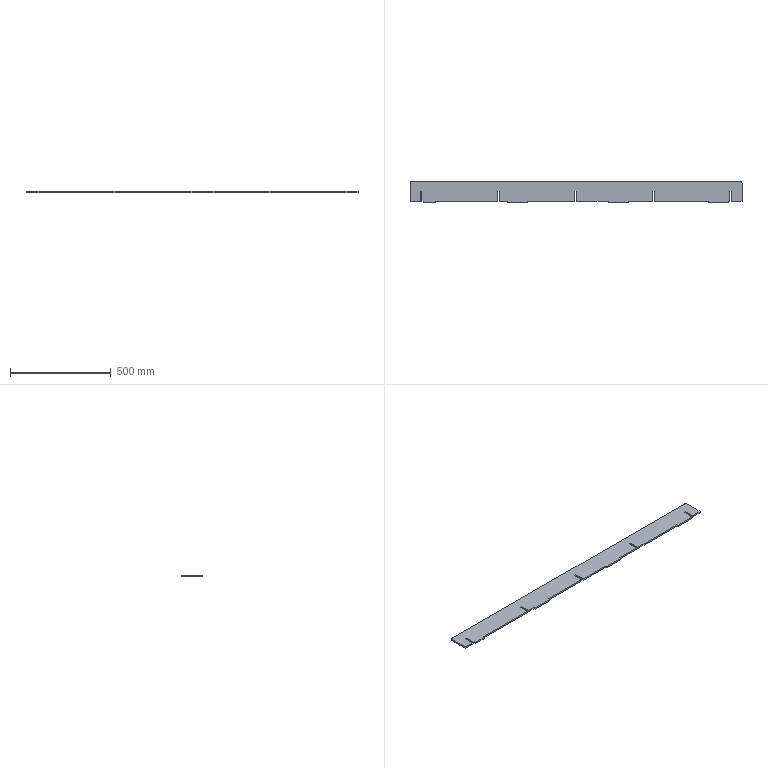Part | SolidWorks | features FlatPattern 1, SMBaseFlange 1, SheetMetal 1 | 1 solid | 44 faces | box 1650 x 107.5 x 8 mm | volume 1325097 mm3 | plane 42 | cylinder 2 | commonest cylinder face diameters 20 x2
STEP:
#1=CARTESIAN_POINT('',(-888.136,168.984,0.));
#2=VERTEX_POINT('',#1);
#3=CARTESIAN_POINT('',(-838.136,168.984,0.));
#4=VERTEX_POINT('',#3);
#5=CARTESIAN_POINT('',(-838.136,168.984,0.));
#6=DIRECTION('',(1.,0.,0.));
#7=VECTOR('',#6,1000.);
#8=LINE('',#5,#7);
#9=EDGE_CURVE('',#2,#4,#8,.T.);
#10=ORIENTED_EDGE('',*,*,#9,.T.);
#11=CARTESIAN_POINT('',(-838.136,168.984,8.));
#12=VERTEX_POINT('',#11);
#13=CARTESIAN_POINT('',(-838.136,168.984,8.));
#14=DIRECTION('',(0.,0.,-1.));
#15=VECTOR('',#14,1000.);
#16=LINE('',#13,#15);
#17=EDGE_CURVE('',#12,#4,#16,.T.);
#18=ORIENTED_EDGE('',*,*,#17,.F.);
#19=CARTESIAN_POINT('',(-888.136,168.984,8.));
#20=VERTEX_POINT('',#19);
#21=CARTESIAN_POINT('',(-838.136,168.984,8.));
#22=DIRECTION('',(1.,0.,0.));
#23=VECTOR('',#22,1000.);
#24=LINE('',#21,#23);
#25=EDGE_CURVE('',#20,#12,#24,.T.);
#26=ORIENTED_EDGE('',*,*,#25,.F.);
#27=CARTESIAN_POINT('',(-888.136,168.984,8.));
#28=DIRECTION('',(0.,0.,-1.));
#29=VECTOR('',#28,1000.);
#30=LINE('',#27,#29);
#31=EDGE_CURVE('',#20,#2,#30,.T.);
#32=ORIENTED_EDGE('',*,*,#31,.T.);
#33=EDGE_LOOP('',(#10,#18,#26,#32));
#34=FACE_OUTER_BOUND('',#33,.T.);
#35=CARTESIAN_POINT('',(-838.136,168.984,8.));
#36=DIRECTION('',(0.,1.,0.));
#37=DIRECTION('',(-1.,0.,0.));
#38=AXIS2_PLACEMENT_3D('',#35,#36,#37);
#39=PLANE('',#38);
#40=ADVANCED_FACE('',(#34),#39,.F.);
#41=CARTESIAN_POINT('',(-838.136,219.484,0.));
#42=VERTEX_POINT('',#41);
#43=CARTESIAN_POINT('',(-838.136,168.984,0.));
#44=DIRECTION('',(0.,1.,0.));
#45=VECTOR('',#44,1000.);
#46=LINE('',#43,#45);
#47=EDGE_CURVE('',#4,#42,#46,.T.);
#48=ORIENTED_EDGE('',*,*,#47,.T.);
#49=CARTESIAN_POINT('',(-838.136,219.484,8.));
#50=VERTEX_POINT('',#49);
#51=CARTESIAN_POINT('',(-838.136,219.484,8.));
#52=DIRECTION('',(0.,0.,-1.));
#53=VECTOR('',#52,1000.);
#54=LINE('',#51,#53);
#55=EDGE_CURVE('',#50,#42,#54,.T.);
#56=ORIENTED_EDGE('',*,*,#55,.F.);
#57=CARTESIAN_POINT('',(-838.136,168.984,8.));
#58=DIRECTION('',(0.,1.,0.));
#59=VECTOR('',#58,1000.);
#60=LINE('',#57,#59);
#61=EDGE_CURVE('',#12,#50,#60,.T.);
#62=ORIENTED_EDGE('',*,*,#61,.F.);
#63=ORIENTED_EDGE('',*,*,#17,.T.);
#64=EDGE_LOOP('',(#48,#56,#62,#63));
#65=FACE_OUTER_BOUND('',#64,.T.);
#66=CARTESIAN_POINT('',(-838.136,168.984,8.));
#67=DIRECTION('',(-1.,0.,0.));
#68=DIRECTION('',(0.,0.,1.));
#69=AXIS2_PLACEMENT_3D('',#66,#67,#68);
#70=PLANE('',#69);
#71=ADVANCED_FACE('',(#65),#70,.F.);
#72=CARTESIAN_POINT('',(-830.136,219.484,0.));
#73=VERTEX_POINT('',#72);
#74=CARTESIAN_POINT('',(-838.136,219.484,0.));
#75=DIRECTION('',(1.,0.,0.));
#76=VECTOR('',#75,1000.);
#77=LINE('',#74,#76);
#78=EDGE_CURVE('',#42,#73,#77,.T.);
#79=ORIENTED_EDGE('',*,*,#78,.T.);
#80=CARTESIAN_POINT('',(-830.136,219.484,8.));
#81=VERTEX_POINT('',#80);
#82=CARTESIAN_POINT('',(-830.136,219.484,8.));
#83=DIRECTION('',(0.,0.,-1.));
#84=VECTOR('',#83,1000.);
#85=LINE('',#82,#84);
#86=EDGE_CURVE('',#81,#73,#85,.T.);
#87=ORIENTED_EDGE('',*,*,#86,.F.);
#88=CARTESIAN_POINT('',(-838.136,219.484,8.));
#89=DIRECTION('',(1.,0.,0.));
#90=VECTOR('',#89,1000.);
#91=LINE('',#88,#90);
#92=EDGE_CURVE('',#50,#81,#91,.T.);
#93=ORIENTED_EDGE('',*,*,#92,.F.);
#94=ORIENTED_EDGE('',*,*,#55,.T.);
#95=EDGE_LOOP('',(#79,#87,#93,#94));
#96=FACE_OUTER_BOUND('',#95,.T.);
#97=CARTESIAN_POINT('',(-838.136,219.484,8.));
#98=DIRECTION('',(0.,1.,0.));
#99=DIRECTION('',(0.,0.,1.));
#100=AXIS2_PLACEMENT_3D('',#97,#98,#99);
#101=PLANE('',#100);
#102=ADVANCED_FACE('',(#96),#101,.F.);
#103=CARTESIAN_POINT('',(-830.136,168.984,0.));
#104=VERTEX_POINT('',#103);
#105=CARTESIAN_POINT('',(-830.136,219.484,0.));
#106=DIRECTION('',(0.,-1.,0.));
#107=VECTOR('',#106,1000.);
#108=LINE('',#105,#107);
#109=EDGE_CURVE('',#73,#104,#108,.T.);
#110=ORIENTED_EDGE('',*,*,#109,.T.);
#111=CARTESIAN_POINT('',(-830.136,168.984,8.));
#112=VERTEX_POINT('',#111);
#113=CARTESIAN_POINT('',(-830.136,168.984,8.));
#114=DIRECTION('',(0.,0.,-1.));
#115=VECTOR('',#114,1000.);
#116=LINE('',#113,#115);
#117=EDGE_CURVE('',#112,#104,#116,.T.);
#118=ORIENTED_EDGE('',*,*,#117,.F.);
#119=CARTESIAN_POINT('',(-830.136,219.484,8.));
#120=DIRECTION('',(0.,-1.,0.));
#121=VECTOR('',#120,1000.);
#122=LINE('',#119,#121);
#123=EDGE_CURVE('',#81,#112,#122,.T.);
#124=ORIENTED_EDGE('',*,*,#123,.F.);
#125=ORIENTED_EDGE('',*,*,#86,.T.);
#126=EDGE_LOOP('',(#110,#118,#124,#125));
#127=FACE_OUTER_BOUND('',#126,.T.);
#128=CARTESIAN_POINT('',(-830.136,219.484,8.));
#129=DIRECTION('',(1.,0.,0.));
#130=DIRECTION('',(0.,0.,-1.));
#131=AXIS2_PLACEMENT_3D('',#128,#129,#130);
#132=PLANE('',#131);
#133=ADVANCED_FACE('',(#127),#132,.F.);
#134=CARTESIAN_POINT('',(-823.136,168.984,0.));
#135=VERTEX_POINT('',#134);
#136=CARTESIAN_POINT('',(-823.136,168.984,0.));
#137=DIRECTION('',(1.,0.,0.));
#138=VECTOR('',#137,1000.);
#139=LINE('',#136,#138);
#140=EDGE_CURVE('',#104,#135,#139,.T.);
#141=ORIENTED_EDGE('',*,*,#140,.T.);
#142=CARTESIAN_POINT('',(-823.136,168.984,8.));
#143=VERTEX_POINT('',#142);
#144=CARTESIAN_POINT('',(-823.136,168.984,8.));
#145=DIRECTION('',(0.,0.,-1.));
#146=VECTOR('',#145,1000.);
#147=LINE('',#144,#146);
#148=EDGE_CURVE('',#143,#135,#147,.T.);
#149=ORIENTED_EDGE('',*,*,#148,.F.);
#150=CARTESIAN_POINT('',(-823.136,168.984,8.));
#151=DIRECTION('',(1.,0.,0.));
#152=VECTOR('',#151,1000.);
#153=LINE('',#150,#152);
#154=EDGE_CURVE('',#112,#143,#153,.T.);
#155=ORIENTED_EDGE('',*,*,#154,.F.);
#156=ORIENTED_EDGE('',*,*,#117,.T.);
#157=EDGE_LOOP('',(#141,#149,#155,#156));
#158=FACE_OUTER_BOUND('',#157,.T.);
#159=CARTESIAN_POINT('',(-823.136,168.984,8.));
#160=DIRECTION('',(0.,1.,0.));
#161=DIRECTION('',(0.,0.,1.));
#162=AXIS2_PLACEMENT_3D('',#159,#160,#161);
#163=PLANE('',#162);
#164=ADVANCED_FACE('',(#158),#163,.F.);
#165=CARTESIAN_POINT('',(-823.136,161.484,0.));
#166=VERTEX_POINT('',#165);
#167=CARTESIAN_POINT('',(-823.136,161.484,0.));
#168=DIRECTION('',(0.,-1.,0.));
#169=VECTOR('',#168,1000.);
#170=LINE('',#167,#169);
#171=EDGE_CURVE('',#135,#166,#170,.T.);
#172=ORIENTED_EDGE('',*,*,#171,.T.);
#173=CARTESIAN_POINT('',(-823.136,161.484,8.));
#174=VERTEX_POINT('',#173);
#175=CARTESIAN_POINT('',(-823.136,161.484,8.));
#176=DIRECTION('',(0.,0.,-1.));
#177=VECTOR('',#176,1000.);
#178=LINE('',#175,#177);
#179=EDGE_CURVE('',#174,#166,#178,.T.);
#180=ORIENTED_EDGE('',*,*,#179,.F.);
#181=CARTESIAN_POINT('',(-823.136,161.484,8.));
#182=DIRECTION('',(0.,-1.,0.));
#183=VECTOR('',#182,1000.);
#184=LINE('',#181,#183);
#185=EDGE_CURVE('',#143,#174,#184,.T.);
#186=ORIENTED_EDGE('',*,*,#185,.F.);
#187=ORIENTED_EDGE('',*,*,#148,.T.);
#188=EDGE_LOOP('',(#172,#180,#186,#187));
#189=FACE_OUTER_BOUND('',#188,.T.);
#190=CARTESIAN_POINT('',(-823.136,161.484,8.));
#191=DIRECTION('',(1.,0.,0.));
#192=DIRECTION('',(0.,0.,-1.));
#193=AXIS2_PLACEMENT_3D('',#190,#191,#192);
#194=PLANE('',#193);
#195=ADVANCED_FACE('',(#189),#194,.F.);
#196=CARTESIAN_POINT('',(-763.136,161.484,0.));
#197=VERTEX_POINT('',#196);
#198=CARTESIAN_POINT('',(-763.136,161.484,0.));
#199=DIRECTION('',(1.,0.,0.));
#200=VECTOR('',#199,1000.);
#201=LINE('',#198,#200);
#202=EDGE_CURVE('',#166,#197,#201,.T.);
#203=ORIENTED_EDGE('',*,*,#202,.T.);
#204=CARTESIAN_POINT('',(-763.136,161.484,8.));
#205=VERTEX_POINT('',#204);
#206=CARTESIAN_POINT('',(-763.136,161.484,8.));
#207=DIRECTION('',(0.,0.,-1.));
#208=VECTOR('',#207,1000.);
#209=LINE('',#206,#208);
#210=EDGE_CURVE('',#205,#197,#209,.T.);
#211=ORIENTED_EDGE('',*,*,#210,.F.);
#212=CARTESIAN_POINT('',(-763.136,161.484,8.));
#213=DIRECTION('',(1.,0.,0.));
#214=VECTOR('',#213,1000.);
#215=LINE('',#212,#214);
#216=EDGE_CURVE('',#174,#205,#215,.T.);
#217=ORIENTED_EDGE('',*,*,#216,.F.);
#218=ORIENTED_EDGE('',*,*,#179,.T.);
#219=EDGE_LOOP('',(#203,#211,#217,#218));
#220=FACE_OUTER_BOUND('',#219,.T.);
#221=CARTESIAN_POINT('',(-763.136,161.484,8.));
#222=DIRECTION('',(0.,1.,0.));
#223=DIRECTION('',(-1.,0.,0.));
#224=AXIS2_PLACEMENT_3D('',#221,#222,#223);
#225=PLANE('',#224);
#226=ADVANCED_FACE('',(#220),#225,.F.);
#227=CARTESIAN_POINT('',(-763.136,168.984,0.));
#228=VERTEX_POINT('',#227);
#229=CARTESIAN_POINT('',(-763.136,168.984,0.));
#230=DIRECTION('',(0.,1.,0.));
#231=VECTOR('',#230,1000.);
#232=LINE('',#229,#231);
#233=EDGE_CURVE('',#197,#228,#232,.T.);
#234=ORIENTED_EDGE('',*,*,#233,.T.);
#235=CARTESIAN_POINT('',(-763.136,168.984,8.));
#236=VERTEX_POINT('',#235);
#237=CARTESIAN_POINT('',(-763.136,168.984,8.));
#238=DIRECTION('',(0.,0.,-1.));
#239=VECTOR('',#238,1000.);
#240=LINE('',#237,#239);
#241=EDGE_CURVE('',#236,#228,#240,.T.);
#242=ORIENTED_EDGE('',*,*,#241,.F.);
#243=CARTESIAN_POINT('',(-763.136,168.984,8.));
#244=DIRECTION('',(0.,1.,0.));
#245=VECTOR('',#244,1000.);
#246=LINE('',#243,#245);
#247=EDGE_CURVE('',#205,#236,#246,.T.);
#248=ORIENTED_EDGE('',*,*,#247,.F.);
#249=ORIENTED_EDGE('',*,*,#210,.T.);
#250=EDGE_LOOP('',(#234,#242,#248,#249));
#251=FACE_OUTER_BOUND('',#250,.T.);
#252=CARTESIAN_POINT('',(-763.136,168.984,8.));
#253=DIRECTION('',(-1.,0.,0.));
#254=DIRECTION('',(0.,0.,1.));
#255=AXIS2_PLACEMENT_3D('',#252,#253,#254);
#256=PLANE('',#255);
#257=ADVANCED_FACE('',(#251),#256,.F.);
#258=CARTESIAN_POINT('',(-453.136,168.984,0.));
#259=VERTEX_POINT('',#258);
#260=CARTESIAN_POINT('',(-453.136,168.984,0.));
#261=DIRECTION('',(1.,0.,0.));
#262=VECTOR('',#261,1000.);
#263=LINE('',#260,#262);
#264=EDGE_CURVE('',#228,#259,#263,.T.);
#265=ORIENTED_EDGE('',*,*,#264,.T.);
#266=CARTESIAN_POINT('',(-453.136,168.984,8.));
#267=VERTEX_POINT('',#266);
#268=CARTESIAN_POINT('',(-453.136,168.984,8.));
#269=DIRECTION('',(0.,0.,-1.));
#270=VECTOR('',#269,1000.);
#271=LINE('',#268,#270);
#272=EDGE_CURVE('',#267,#259,#271,.T.);
#273=ORIENTED_EDGE('',*,*,#272,.F.);
#274=CARTESIAN_POINT('',(-453.136,168.984,8.));
#275=DIRECTION('',(1.,0.,0.));
#276=VECTOR('',#275,1000.);
#277=LINE('',#274,#276);
#278=EDGE_CURVE('',#236,#267,#277,.T.);
#279=ORIENTED_EDGE('',*,*,#278,.F.);
#280=ORIENTED_EDGE('',*,*,#241,.T.);
#281=EDGE_LOOP('',(#265,#273,#279,#280));
#282=FACE_OUTER_BOUND('',#281,.T.);
#283=CARTESIAN_POINT('',(-453.136,168.984,8.));
#284=DIRECTION('',(0.,1.,0.));
#285=DIRECTION('',(-1.,0.,0.));
#286=AXIS2_PLACEMENT_3D('',#283,#284,#285);
#287=PLANE('',#286);
#288=ADVANCED_FACE('',(#282),#287,.F.);
#289=CARTESIAN_POINT('',(-453.136,219.484,0.));
#290=VERTEX_POINT('',#289);
#291=CARTESIAN_POINT('',(-453.136,168.984,0.));
#292=DIRECTION('',(0.,1.,0.));
#293=VECTOR('',#292,1000.);
#294=LINE('',#291,#293);
#295=EDGE_CURVE('',#259,#290,#294,.T.);
#296=ORIENTED_EDGE('',*,*,#295,.T.);
#297=CARTESIAN_POINT('',(-453.136,219.484,8.));
#298=VERTEX_POINT('',#297);
#299=CARTESIAN_POINT('',(-453.136,219.484,8.));
#300=DIRECTION('',(0.,0.,-1.));
#301=VECTOR('',#300,1000.);
#302=LINE('',#299,#301);
#303=EDGE_CURVE('',#298,#290,#302,.T.);
#304=ORIENTED_EDGE('',*,*,#303,.F.);
#305=CARTESIAN_POINT('',(-453.136,168.984,8.));
#306=DIRECTION('',(0.,1.,0.));
#307=VECTOR('',#306,1000.);
#308=LINE('',#305,#307);
#309=EDGE_CURVE('',#267,#298,#308,.T.);
#310=ORIENTED_EDGE('',*,*,#309,.F.);
#311=ORIENTED_EDGE('',*,*,#272,.T.);
#312=EDGE_LOOP('',(#296,#304,#310,#311));
#313=FACE_OUTER_BOUND('',#312,.T.);
#314=CARTESIAN_POINT('',(-453.136,168.984,8.));
#315=DIRECTION('',(-1.,0.,0.));
#316=DIRECTION('',(0.,0.,1.));
#317=AXIS2_PLACEMENT_3D('',#314,#315,#316);
#318=PLANE('',#317);
#319=ADVANCED_FACE('',(#313),#318,.F.);
#320=CARTESIAN_POINT('',(-445.136,219.484,0.));
#321=VERTEX_POINT('',#320);
#322=CARTESIAN_POINT('',(-453.136,219.484,0.));
#323=DIRECTION('',(1.,0.,0.));
#324=VECTOR('',#323,1000.);
#325=LINE('',#322,#324);
#326=EDGE_CURVE('',#290,#321,#325,.T.);
#327=ORIENTED_EDGE('',*,*,#326,.T.);
#328=CARTESIAN_POINT('',(-445.136,219.484,8.));
#329=VERTEX_POINT('',#328);
#330=CARTESIAN_POINT('',(-445.136,219.484,8.));
#331=DIRECTION('',(0.,0.,-1.));
#332=VECTOR('',#331,1000.);
#333=LINE('',#330,#332);
#334=EDGE_CURVE('',#329,#321,#333,.T.);
#335=ORIENTED_EDGE('',*,*,#334,.F.);
#336=CARTESIAN_POINT('',(-453.136,219.484,8.));
#337=DIRECTION('',(1.,0.,0.));
#338=VECTOR('',#337,1000.);
#339=LINE('',#336,#338);
#340=EDGE_CURVE('',#298,#329,#339,.T.);
#341=ORIENTED_EDGE('',*,*,#340,.F.);
#342=ORIENTED_EDGE('',*,*,#303,.T.);
#343=EDGE_LOOP('',(#327,#335,#341,#342));
#344=FACE_OUTER_BOUND('',#343,.T.);
#345=CARTESIAN_POINT('',(-453.136,219.484,8.));
#346=DIRECTION('',(0.,1.,0.));
#347=DIRECTION('',(0.,0.,1.));
#348=AXIS2_PLACEMENT_3D('',#345,#346,#347);
#349=PLANE('',#348);
#350=ADVANCED_FACE('',(#344),#349,.F.);
#351=CARTESIAN_POINT('',(-445.136,168.984,0.));
#352=VERTEX_POINT('',#351);
#353=CARTESIAN_POINT('',(-445.136,219.484,0.));
#354=DIRECTION('',(0.,-1.,0.));
#355=VECTOR('',#354,1000.);
#356=LINE('',#353,#355);
#357=EDGE_CURVE('',#321,#352,#356,.T.);
#358=ORIENTED_EDGE('',*,*,#357,.T.);
#359=CARTESIAN_POINT('',(-445.136,168.984,8.));
#360=VERTEX_POINT('',#359);
#361=CARTESIAN_POINT('',(-445.136,168.984,8.));
#362=DIRECTION('',(0.,0.,-1.));
#363=VECTOR('',#362,1000.);
#364=LINE('',#361,#363);
#365=EDGE_CURVE('',#360,#352,#364,.T.);
#366=ORIENTED_EDGE('',*,*,#365,.F.);
#367=CARTESIAN_POINT('',(-445.136,219.484,8.));
#368=DIRECTION('',(0.,-1.,0.));
#369=VECTOR('',#368,1000.);
#370=LINE('',#367,#369);
#371=EDGE_CURVE('',#329,#360,#370,.T.);
#372=ORIENTED_EDGE('',*,*,#371,.F.);
#373=ORIENTED_EDGE('',*,*,#334,.T.);
#374=EDGE_LOOP('',(#358,#366,#372,#373));
#375=FACE_OUTER_BOUND('',#374,.T.);
#376=CARTESIAN_POINT('',(-445.136,219.484,8.));
#377=DIRECTION('',(1.,0.,0.));
#378=DIRECTION('',(0.,0.,-1.));
#379=AXIS2_PLACEMENT_3D('',#376,#377,#378);
#380=PLANE('',#379);
#381=ADVANCED_FACE('',(#375),#380,.F.);
#382=CARTESIAN_POINT('',(-403.136,168.984,0.));
#383=VERTEX_POINT('',#382);
#384=CARTESIAN_POINT('',(-403.136,168.984,0.));
#385=DIRECTION('',(1.,0.,0.));
#386=VECTOR('',#385,1000.);
#387=LINE('',#384,#386);
#388=EDGE_CURVE('',#352,#383,#387,.T.);
#389=ORIENTED_EDGE('',*,*,#388,.T.);
#390=CARTESIAN_POINT('',(-403.136,168.984,8.));
#391=VERTEX_POINT('',#390);
#392=CARTESIAN_POINT('',(-403.136,168.984,8.));
#393=DIRECTION('',(0.,0.,-1.));
#394=VECTOR('',#393,1000.);
#395=LINE('',#392,#394);
#396=EDGE_CURVE('',#391,#383,#395,.T.);
#397=ORIENTED_EDGE('',*,*,#396,.F.);
#398=CARTESIAN_POINT('',(-403.136,168.984,8.));
#399=DIRECTION('',(1.,0.,0.));
#400=VECTOR('',#399,1000.);
#401=LINE('',#398,#400);
#402=EDGE_CURVE('',#360,#391,#401,.T.);
#403=ORIENTED_EDGE('',*,*,#402,.F.);
#404=ORIENTED_EDGE('',*,*,#365,.T.);
#405=EDGE_LOOP('',(#389,#397,#403,#404));
#406=FACE_OUTER_BOUND('',#405,.T.);
#407=CARTESIAN_POINT('',(-403.136,168.984,8.));
#408=DIRECTION('',(0.,1.,0.));
#409=DIRECTION('',(0.,0.,1.));
#410=AXIS2_PLACEMENT_3D('',#407,#408,#409);
#411=PLANE('',#410);
#412=ADVANCED_FACE('',(#406),#411,.F.);
#413=CARTESIAN_POINT('',(-403.136,161.484,0.));
#414=VERTEX_POINT('',#413);
#415=CARTESIAN_POINT('',(-403.136,161.484,0.));
#416=DIRECTION('',(0.,-1.,0.));
#417=VECTOR('',#416,1000.);
#418=LINE('',#415,#417);
#419=EDGE_CURVE('',#383,#414,#418,.T.);
#420=ORIENTED_EDGE('',*,*,#419,.T.);
#421=CARTESIAN_POINT('',(-403.136,161.484,8.));
#422=VERTEX_POINT('',#421);
#423=CARTESIAN_POINT('',(-403.136,161.484,8.));
#424=DIRECTION('',(0.,0.,-1.));
#425=VECTOR('',#424,1000.);
#426=LINE('',#423,#425);
#427=EDGE_CURVE('',#422,#414,#426,.T.);
#428=ORIENTED_EDGE('',*,*,#427,.F.);
#429=CARTESIAN_POINT('',(-403.136,161.484,8.));
#430=DIRECTION('',(0.,-1.,0.));
#431=VECTOR('',#430,1000.);
#432=LINE('',#429,#431);
#433=EDGE_CURVE('',#391,#422,#432,.T.);
#434=ORIENTED_EDGE('',*,*,#433,.F.);
#435=ORIENTED_EDGE('',*,*,#396,.T.);
#436=EDGE_LOOP('',(#420,#428,#434,#435));
#437=FACE_OUTER_BOUND('',#436,.T.);
#438=CARTESIAN_POINT('',(-403.136,161.484,8.));
#439=DIRECTION('',(1.,0.,0.));
#440=DIRECTION('',(0.,0.,-1.));
#441=AXIS2_PLACEMENT_3D('',#438,#439,#440);
#442=PLANE('',#441);
#443=ADVANCED_FACE('',(#437),#442,.F.);
#444=CARTESIAN_POINT('',(-303.136,161.484,0.));
#445=VERTEX_POINT('',#444);
#446=CARTESIAN_POINT('',(-303.136,161.484,0.));
#447=DIRECTION('',(1.,0.,0.));
#448=VECTOR('',#447,1000.);
#449=LINE('',#446,#448);
#450=EDGE_CURVE('',#414,#445,#449,.T.);
#451=ORIENTED_EDGE('',*,*,#450,.T.);
#452=CARTESIAN_POINT('',(-303.136,161.484,8.));
#453=VERTEX_POINT('',#452);
#454=CARTESIAN_POINT('',(-303.136,161.484,8.));
#455=DIRECTION('',(0.,0.,-1.));
#456=VECTOR('',#455,1000.);
#457=LINE('',#454,#456);
#458=EDGE_CURVE('',#453,#445,#457,.T.);
#459=ORIENTED_EDGE('',*,*,#458,.F.);
#460=CARTESIAN_POINT('',(-303.136,161.484,8.));
#461=DIRECTION('',(1.,0.,0.));
#462=VECTOR('',#461,1000.);
#463=LINE('',#460,#462);
#464=EDGE_CURVE('',#422,#453,#463,.T.);
#465=ORIENTED_EDGE('',*,*,#464,.F.);
#466=ORIENTED_EDGE('',*,*,#427,.T.);
#467=EDGE_LOOP('',(#451,#459,#465,#466));
#468=FACE_OUTER_BOUND('',#467,.T.);
#469=CARTESIAN_POINT('',(-303.136,161.484,8.));
#470=DIRECTION('',(0.,1.,0.));
#471=DIRECTION('',(-1.,0.,0.));
#472=AXIS2_PLACEMENT_3D('',#469,#470,#471);
#473=PLANE('',#472);
#474=ADVANCED_FACE('',(#468),#473,.F.);
#475=CARTESIAN_POINT('',(-303.136,168.984,0.));
#476=VERTEX_POINT('',#475);
#477=CARTESIAN_POINT('',(-303.136,168.984,0.));
#478=DIRECTION('',(0.,1.,0.));
#479=VECTOR('',#478,1000.);
#480=LINE('',#477,#479);
#481=EDGE_CURVE('',#445,#476,#480,.T.);
#482=ORIENTED_EDGE('',*,*,#481,.T.);
#483=CARTESIAN_POINT('',(-303.136,168.984,8.));
#484=VERTEX_POINT('',#483);
#485=CARTESIAN_POINT('',(-303.136,168.984,8.));
#486=DIRECTION('',(0.,0.,-1.));
#487=VECTOR('',#486,1000.);
#488=LINE('',#485,#487);
#489=EDGE_CURVE('',#484,#476,#488,.T.);
#490=ORIENTED_EDGE('',*,*,#489,.F.);
#491=CARTESIAN_POINT('',(-303.136,168.984,8.));
#492=DIRECTION('',(0.,1.,0.));
#493=VECTOR('',#492,1000.);
#494=LINE('',#491,#493);
#495=EDGE_CURVE('',#453,#484,#494,.T.);
#496=ORIENTED_EDGE('',*,*,#495,.F.);
#497=ORIENTED_EDGE('',*,*,#458,.T.);
#498=EDGE_LOOP('',(#482,#490,#496,#497));
#499=FACE_OUTER_BOUND('',#498,.T.);
#500=CARTESIAN_POINT('',(-303.136,168.984,8.));
#501=DIRECTION('',(-1.,0.,0.));
#502=DIRECTION('',(0.,0.,1.));
#503=AXIS2_PLACEMENT_3D('',#500,#501,#502);
#504=PLANE('',#503);
#505=ADVANCED_FACE('',(#499),#504,.F.);
#506=CARTESIAN_POINT('',(-68.136,168.984,0.));
#507=VERTEX_POINT('',#506);
#508=CARTESIAN_POINT('',(-68.136,168.984,0.));
#509=DIRECTION('',(1.,0.,0.));
#510=VECTOR('',#509,1000.);
#511=LINE('',#508,#510);
#512=EDGE_CURVE('',#476,#507,#511,.T.);
#513=ORIENTED_EDGE('',*,*,#512,.T.);
#514=CARTESIAN_POINT('',(-68.136,168.984,8.));
#515=VERTEX_POINT('',#514);
#516=CARTESIAN_POINT('',(-68.136,168.984,8.));
#517=DIRECTION('',(0.,0.,-1.));
#518=VECTOR('',#517,1000.);
#519=LINE('',#516,#518);
#520=EDGE_CURVE('',#515,#507,#519,.T.);
#521=ORIENTED_EDGE('',*,*,#520,.F.);
#522=CARTESIAN_POINT('',(-68.136,168.984,8.));
#523=DIRECTION('',(1.,0.,0.));
#524=VECTOR('',#523,1000.);
#525=LINE('',#522,#524);
#526=EDGE_CURVE('',#484,#515,#525,.T.);
#527=ORIENTED_EDGE('',*,*,#526,.F.);
#528=ORIENTED_EDGE('',*,*,#489,.T.);
#529=EDGE_LOOP('',(#513,#521,#527,#528));
#530=FACE_OUTER_BOUND('',#529,.T.);
#531=CARTESIAN_POINT('',(-68.136,168.984,8.));
#532=DIRECTION('',(0.,1.,0.));
#533=DIRECTION('',(-1.,0.,0.));
#534=AXIS2_PLACEMENT_3D('',#531,#532,#533);
#535=PLANE('',#534);
#536=ADVANCED_FACE('',(#530),#535,.F.);
#537=CARTESIAN_POINT('',(-68.136,219.484,0.));
#538=VERTEX_POINT('',#537);
#539=CARTESIAN_POINT('',(-68.136,168.984,0.));
#540=DIRECTION('',(0.,1.,0.));
#541=VECTOR('',#540,1000.);
#542=LINE('',#539,#541);
#543=EDGE_CURVE('',#507,#538,#542,.T.);
#544=ORIENTED_EDGE('',*,*,#543,.T.);
#545=CARTESIAN_POINT('',(-68.136,219.484,8.));
#546=VERTEX_POINT('',#545);
#547=CARTESIAN_POINT('',(-68.136,219.484,8.));
#548=DIRECTION('',(0.,0.,-1.));
#549=VECTOR('',#548,1000.);
#550=LINE('',#547,#549);
#551=EDGE_CURVE('',#546,#538,#550,.T.);
#552=ORIENTED_EDGE('',*,*,#551,.F.);
#553=CARTESIAN_POINT('',(-68.136,168.984,8.));
#554=DIRECTION('',(0.,1.,0.));
#555=VECTOR('',#554,1000.);
#556=LINE('',#553,#555);
#557=EDGE_CURVE('',#515,#546,#556,.T.);
#558=ORIENTED_EDGE('',*,*,#557,.F.);
#559=ORIENTED_EDGE('',*,*,#520,.T.);
#560=EDGE_LOOP('',(#544,#552,#558,#559));
#561=FACE_OUTER_BOUND('',#560,.T.);
#562=CARTESIAN_POINT('',(-68.136,168.984,8.));
#563=DIRECTION('',(-1.,0.,0.));
#564=DIRECTION('',(0.,0.,1.));
#565=AXIS2_PLACEMENT_3D('',#562,#563,#564);
#566=PLANE('',#565);
#567=ADVANCED_FACE('',(#561),#566,.F.);
#568=CARTESIAN_POINT('',(-60.136,219.484,0.));
#569=VERTEX_POINT('',#568);
#570=CARTESIAN_POINT('',(-68.136,219.484,0.));
#571=DIRECTION('',(1.,0.,0.));
#572=VECTOR('',#571,1000.);
#573=LINE('',#570,#572);
#574=EDGE_CURVE('',#538,#569,#573,.T.);
#575=ORIENTED_EDGE('',*,*,#574,.T.);
#576=CARTESIAN_POINT('',(-60.136,219.484,8.));
#577=VERTEX_POINT('',#576);
#578=CARTESIAN_POINT('',(-60.136,219.484,8.));
#579=DIRECTION('',(0.,0.,-1.));
#580=VECTOR('',#579,1000.);
#581=LINE('',#578,#580);
#582=EDGE_CURVE('',#577,#569,#581,.T.);
#583=ORIENTED_EDGE('',*,*,#582,.F.);
#584=CARTESIAN_POINT('',(-68.136,219.484,8.));
#585=DIRECTION('',(1.,0.,0.));
#586=VECTOR('',#585,1000.);
#587=LINE('',#584,#586);
#588=EDGE_CURVE('',#546,#577,#587,.T.);
#589=ORIENTED_EDGE('',*,*,#588,.F.);
#590=ORIENTED_EDGE('',*,*,#551,.T.);
#591=EDGE_LOOP('',(#575,#583,#589,#590));
#592=FACE_OUTER_BOUND('',#591,.T.);
#593=CARTESIAN_POINT('',(-68.136,219.484,8.));
#594=DIRECTION('',(0.,1.,0.));
#595=DIRECTION('',(0.,0.,1.));
#596=AXIS2_PLACEMENT_3D('',#593,#594,#595);
#597=PLANE('',#596);
#598=ADVANCED_FACE('',(#592),#597,.F.);
#599=CARTESIAN_POINT('',(-60.136,168.984,0.));
#600=VERTEX_POINT('',#599);
#601=CARTESIAN_POINT('',(-60.136,219.484,0.));
#602=DIRECTION('',(0.,-1.,0.));
#603=VECTOR('',#602,1000.);
#604=LINE('',#601,#603);
#605=EDGE_CURVE('',#569,#600,#604,.T.);
#606=ORIENTED_EDGE('',*,*,#605,.T.);
#607=CARTESIAN_POINT('',(-60.136,168.984,8.));
#608=VERTEX_POINT('',#607);
#609=CARTESIAN_POINT('',(-60.136,168.984,8.));
#610=DIRECTION('',(0.,0.,-1.));
#611=VECTOR('',#610,1000.);
#612=LINE('',#609,#611);
#613=EDGE_CURVE('',#608,#600,#612,.T.);
#614=ORIENTED_EDGE('',*,*,#613,.F.);
#615=CARTESIAN_POINT('',(-60.136,219.484,8.));
#616=DIRECTION('',(0.,-1.,0.));
#617=VECTOR('',#616,1000.);
#618=LINE('',#615,#617);
#619=EDGE_CURVE('',#577,#608,#618,.T.);
#620=ORIENTED_EDGE('',*,*,#619,.F.);
#621=ORIENTED_EDGE('',*,*,#582,.T.);
#622=EDGE_LOOP('',(#606,#614,#620,#621));
#623=FACE_OUTER_BOUND('',#622,.T.);
#624=CARTESIAN_POINT('',(-60.136,219.484,8.));
#625=DIRECTION('',(1.,0.,0.));
#626=DIRECTION('',(0.,0.,-1.));
#627=AXIS2_PLACEMENT_3D('',#624,#625,#626);
#628=PLANE('',#627);
#629=ADVANCED_FACE('',(#623),#628,.F.);
#630=CARTESIAN_POINT('',(96.864,168.984,0.));
#631=VERTEX_POINT('',#630);
#632=CARTESIAN_POINT('',(96.864,168.984,0.));
#633=DIRECTION('',(1.,0.,0.));
#634=VECTOR('',#633,1000.);
#635=LINE('',#632,#634);
#636=EDGE_CURVE('',#600,#631,#635,.T.);
#637=ORIENTED_EDGE('',*,*,#636,.T.);
#638=CARTESIAN_POINT('',(96.864,168.984,8.));
#639=VERTEX_POINT('',#638);
#640=CARTESIAN_POINT('',(96.864,168.984,8.));
#641=DIRECTION('',(0.,0.,-1.));
#642=VECTOR('',#641,1000.);
#643=LINE('',#640,#642);
#644=EDGE_CURVE('',#639,#631,#643,.T.);
#645=ORIENTED_EDGE('',*,*,#644,.F.);
#646=CARTESIAN_POINT('',(96.864,168.984,8.));
#647=DIRECTION('',(1.,0.,0.));
#648=VECTOR('',#647,1000.);
#649=LINE('',#646,#648);
#650=EDGE_CURVE('',#608,#639,#649,.T.);
#651=ORIENTED_EDGE('',*,*,#650,.F.);
#652=ORIENTED_EDGE('',*,*,#613,.T.);
#653=EDGE_LOOP('',(#637,#645,#651,#652));
#654=FACE_OUTER_BOUND('',#653,.T.);
#655=CARTESIAN_POINT('',(96.864,168.984,8.));
#656=DIRECTION('',(0.,1.,0.));
#657=DIRECTION('',(0.,0.,1.));
#658=AXIS2_PLACEMENT_3D('',#655,#656,#657);
#659=PLANE('',#658);
#660=ADVANCED_FACE('',(#654),#659,.F.);
#661=CARTESIAN_POINT('',(96.864,161.484,0.));
#662=VERTEX_POINT('',#661);
#663=CARTESIAN_POINT('',(96.864,161.484,0.));
#664=DIRECTION('',(0.,-1.,0.));
#665=VECTOR('',#664,1000.);
#666=LINE('',#663,#665);
#667=EDGE_CURVE('',#631,#662,#666,.T.);
#668=ORIENTED_EDGE('',*,*,#667,.T.);
#669=CARTESIAN_POINT('',(96.864,161.484,8.));
#670=VERTEX_POINT('',#669);
#671=CARTESIAN_POINT('',(96.864,161.484,8.));
#672=DIRECTION('',(0.,0.,-1.));
#673=VECTOR('',#672,1000.);
#674=LINE('',#671,#673);
#675=EDGE_CURVE('',#670,#662,#674,.T.);
#676=ORIENTED_EDGE('',*,*,#675,.F.);
#677=CARTESIAN_POINT('',(96.864,161.484,8.));
#678=DIRECTION('',(0.,-1.,0.));
#679=VECTOR('',#678,1000.);
#680=LINE('',#677,#679);
#681=EDGE_CURVE('',#639,#670,#680,.T.);
#682=ORIENTED_EDGE('',*,*,#681,.F.);
#683=ORIENTED_EDGE('',*,*,#644,.T.);
#684=EDGE_LOOP('',(#668,#676,#682,#683));
#685=FACE_OUTER_BOUND('',#684,.T.);
#686=CARTESIAN_POINT('',(96.864,161.484,8.));
#687=DIRECTION('',(1.,0.,0.));
#688=DIRECTION('',(0.,1.,0.));
#689=AXIS2_PLACEMENT_3D('',#686,#687,#688);
#690=PLANE('',#689);
#691=ADVANCED_FACE('',(#685),#690,.F.);
#692=CARTESIAN_POINT('',(196.864,161.484,0.));
#693=VERTEX_POINT('',#692);
#694=CARTESIAN_POINT('',(196.864,161.484,0.));
#695=DIRECTION('',(1.,0.,0.));
#696=VECTOR('',#695,1000.);
#697=LINE('',#694,#696);
#698=EDGE_CURVE('',#662,#693,#697,.T.);
#699=ORIENTED_EDGE('',*,*,#698,.T.);
#700=CARTESIAN_POINT('',(196.864,161.484,8.));
#701=VERTEX_POINT('',#700);
#702=CARTESIAN_POINT('',(196.864,161.484,8.));
#703=DIRECTION('',(0.,0.,-1.));
#704=VECTOR('',#703,1000.);
#705=LINE('',#702,#704);
#706=EDGE_CURVE('',#701,#693,#705,.T.);
#707=ORIENTED_EDGE('',*,*,#706,.F.);
#708=CARTESIAN_POINT('',(196.864,161.484,8.));
#709=DIRECTION('',(1.,0.,0.));
#710=VECTOR('',#709,1000.);
#711=LINE('',#708,#710);
#712=EDGE_CURVE('',#670,#701,#711,.T.);
#713=ORIENTED_EDGE('',*,*,#712,.F.);
#714=ORIENTED_EDGE('',*,*,#675,.T.);
#715=EDGE_LOOP('',(#699,#707,#713,#714));
#716=FACE_OUTER_BOUND('',#715,.T.);
#717=CARTESIAN_POINT('',(196.864,161.484,8.));
#718=DIRECTION('',(0.,1.,0.));
#719=DIRECTION('',(0.,0.,1.));
#720=AXIS2_PLACEMENT_3D('',#717,#718,#719);
#721=PLANE('',#720);
#722=ADVANCED_FACE('',(#716),#721,.F.);
#723=CARTESIAN_POINT('',(196.864,168.984,0.));
#724=VERTEX_POINT('',#723);
#725=CARTESIAN_POINT('',(196.864,168.984,0.));
#726=DIRECTION('',(0.,1.,0.));
#727=VECTOR('',#726,1000.);
#728=LINE('',#725,#727);
#729=EDGE_CURVE('',#693,#724,#728,.T.);
#730=ORIENTED_EDGE('',*,*,#729,.T.);
#731=CARTESIAN_POINT('',(196.864,168.984,8.));
#732=VERTEX_POINT('',#731);
#733=CARTESIAN_POINT('',(196.864,168.984,8.));
#734=DIRECTION('',(0.,0.,-1.));
#735=VECTOR('',#734,1000.);
#736=LINE('',#733,#735);
#737=EDGE_CURVE('',#732,#724,#736,.T.);
#738=ORIENTED_EDGE('',*,*,#737,.F.);
#739=CARTESIAN_POINT('',(196.864,168.984,8.));
#740=DIRECTION('',(0.,1.,0.));
#741=VECTOR('',#740,1000.);
#742=LINE('',#739,#741);
#743=EDGE_CURVE('',#701,#732,#742,.T.);
#744=ORIENTED_EDGE('',*,*,#743,.F.);
#745=ORIENTED_EDGE('',*,*,#706,.T.);
#746=EDGE_LOOP('',(#730,#738,#744,#745));
#747=FACE_OUTER_BOUND('',#746,.T.);
#748=CARTESIAN_POINT('',(196.864,168.984,8.));
#749=DIRECTION('',(-1.,0.,0.));
#750=DIRECTION('',(0.,0.,1.));
#751=AXIS2_PLACEMENT_3D('',#748,#749,#750);
#752=PLANE('',#751);
#753=ADVANCED_FACE('',(#747),#752,.F.);
#754=CARTESIAN_POINT('',(316.864,168.984,0.));
#755=VERTEX_POINT('',#754);
#756=CARTESIAN_POINT('',(316.864,168.984,0.));
#757=DIRECTION('',(1.,0.,0.));
#758=VECTOR('',#757,1000.);
#759=LINE('',#756,#758);
#760=EDGE_CURVE('',#724,#755,#759,.T.);
#761=ORIENTED_EDGE('',*,*,#760,.T.);
#762=CARTESIAN_POINT('',(316.864,168.984,8.));
#763=VERTEX_POINT('',#762);
#764=CARTESIAN_POINT('',(316.864,168.984,8.));
#765=DIRECTION('',(0.,0.,-1.));
#766=VECTOR('',#765,1000.);
#767=LINE('',#764,#766);
#768=EDGE_CURVE('',#763,#755,#767,.T.);
#769=ORIENTED_EDGE('',*,*,#768,.F.);
#770=CARTESIAN_POINT('',(316.864,168.984,8.));
#771=DIRECTION('',(1.,0.,0.));
#772=VECTOR('',#771,1000.);
#773=LINE('',#770,#772);
#774=EDGE_CURVE('',#732,#763,#773,.T.);
#775=ORIENTED_EDGE('',*,*,#774,.F.);
#776=ORIENTED_EDGE('',*,*,#737,.T.);
#777=EDGE_LOOP('',(#761,#769,#775,#776));
#778=FACE_OUTER_BOUND('',#777,.T.);
#779=CARTESIAN_POINT('',(316.864,168.984,8.));
#780=DIRECTION('',(0.,1.,0.));
#781=DIRECTION('',(-1.,0.,0.));
#782=AXIS2_PLACEMENT_3D('',#779,#780,#781);
#783=PLANE('',#782);
#784=ADVANCED_FACE('',(#778),#783,.F.);
#785=CARTESIAN_POINT('',(316.864,219.484,0.));
#786=VERTEX_POINT('',#785);
#787=CARTESIAN_POINT('',(316.864,168.984,0.));
#788=DIRECTION('',(0.,1.,0.));
#789=VECTOR('',#788,1000.);
#790=LINE('',#787,#789);
#791=EDGE_CURVE('',#755,#786,#790,.T.);
#792=ORIENTED_EDGE('',*,*,#791,.T.);
#793=CARTESIAN_POINT('',(316.864,219.484,8.));
#794=VERTEX_POINT('',#793);
#795=CARTESIAN_POINT('',(316.864,219.484,8.));
#796=DIRECTION('',(0.,0.,-1.));
#797=VECTOR('',#796,1000.);
#798=LINE('',#795,#797);
#799=EDGE_CURVE('',#794,#786,#798,.T.);
#800=ORIENTED_EDGE('',*,*,#799,.F.);
#801=CARTESIAN_POINT('',(316.864,168.984,8.));
#802=DIRECTION('',(0.,1.,0.));
#803=VECTOR('',#802,1000.);
#804=LINE('',#801,#803);
#805=EDGE_CURVE('',#763,#794,#804,.T.);
#806=ORIENTED_EDGE('',*,*,#805,.F.);
#807=ORIENTED_EDGE('',*,*,#768,.T.);
#808=EDGE_LOOP('',(#792,#800,#806,#807));
#809=FACE_OUTER_BOUND('',#808,.T.);
#810=CARTESIAN_POINT('',(316.864,168.984,8.));
#811=DIRECTION('',(-1.,0.,0.));
#812=DIRECTION('',(0.,0.,1.));
#813=AXIS2_PLACEMENT_3D('',#810,#811,#812);
#814=PLANE('',#813);
#815=ADVANCED_FACE('',(#809),#814,.F.);
#816=CARTESIAN_POINT('',(324.864,219.484,0.));
#817=VERTEX_POINT('',#816);
#818=CARTESIAN_POINT('',(316.864,219.484,0.));
#819=DIRECTION('',(1.,0.,0.));
#820=VECTOR('',#819,1000.);
#821=LINE('',#818,#820);
#822=EDGE_CURVE('',#786,#817,#821,.T.);
#823=ORIENTED_EDGE('',*,*,#822,.T.);
#824=CARTESIAN_POINT('',(324.864,219.484,8.));
#825=VERTEX_POINT('',#824);
#826=CARTESIAN_POINT('',(324.864,219.484,8.));
#827=DIRECTION('',(0.,0.,-1.));
#828=VECTOR('',#827,1000.);
#829=LINE('',#826,#828);
#830=EDGE_CURVE('',#825,#817,#829,.T.);
#831=ORIENTED_EDGE('',*,*,#830,.F.);
#832=CARTESIAN_POINT('',(316.864,219.484,8.));
#833=DIRECTION('',(1.,0.,0.));
#834=VECTOR('',#833,1000.);
#835=LINE('',#832,#834);
#836=EDGE_CURVE('',#794,#825,#835,.T.);
#837=ORIENTED_EDGE('',*,*,#836,.F.);
#838=ORIENTED_EDGE('',*,*,#799,.T.);
#839=EDGE_LOOP('',(#823,#831,#837,#838));
#840=FACE_OUTER_BOUND('',#839,.T.);
#841=CARTESIAN_POINT('',(316.864,219.484,8.));
#842=DIRECTION('',(0.,1.,0.));
#843=DIRECTION('',(0.,0.,1.));
#844=AXIS2_PLACEMENT_3D('',#841,#842,#843);
#845=PLANE('',#844);
#846=ADVANCED_FACE('',(#840),#845,.F.);
#847=CARTESIAN_POINT('',(324.864,168.984,0.));
#848=VERTEX_POINT('',#847);
#849=CARTESIAN_POINT('',(324.864,219.484,0.));
#850=DIRECTION('',(0.,-1.,0.));
#851=VECTOR('',#850,1000.);
#852=LINE('',#849,#851);
#853=EDGE_CURVE('',#817,#848,#852,.T.);
#854=ORIENTED_EDGE('',*,*,#853,.T.);
#855=CARTESIAN_POINT('',(324.864,168.984,8.));
#856=VERTEX_POINT('',#855);
#857=CARTESIAN_POINT('',(324.864,168.984,8.));
#858=DIRECTION('',(0.,0.,-1.));
#859=VECTOR('',#858,1000.);
#860=LINE('',#857,#859);
#861=EDGE_CURVE('',#856,#848,#860,.T.);
#862=ORIENTED_EDGE('',*,*,#861,.F.);
#863=CARTESIAN_POINT('',(324.864,219.484,8.));
#864=DIRECTION('',(0.,-1.,0.));
#865=VECTOR('',#864,1000.);
#866=LINE('',#863,#865);
#867=EDGE_CURVE('',#825,#856,#866,.T.);
#868=ORIENTED_EDGE('',*,*,#867,.F.);
#869=ORIENTED_EDGE('',*,*,#830,.T.);
#870=EDGE_LOOP('',(#854,#862,#868,#869));
#871=FACE_OUTER_BOUND('',#870,.T.);
#872=CARTESIAN_POINT('',(324.864,219.484,8.));
#873=DIRECTION('',(1.,0.,0.));
#874=DIRECTION('',(0.,0.,-1.));
#875=AXIS2_PLACEMENT_3D('',#872,#873,#874);
#876=PLANE('',#875);
#877=ADVANCED_FACE('',(#871),#876,.F.);
#878=CARTESIAN_POINT('',(596.864,168.984,0.));
#879=VERTEX_POINT('',#878);
#880=CARTESIAN_POINT('',(596.864,168.984,0.));
#881=DIRECTION('',(1.,0.,0.));
#882=VECTOR('',#881,1000.);
#883=LINE('',#880,#882);
#884=EDGE_CURVE('',#848,#879,#883,.T.);
#885=ORIENTED_EDGE('',*,*,#884,.T.);
#886=CARTESIAN_POINT('',(596.864,168.984,8.));
#887=VERTEX_POINT('',#886);
#888=CARTESIAN_POINT('',(596.864,168.984,8.));
#889=DIRECTION('',(0.,0.,-1.));
#890=VECTOR('',#889,1000.);
#891=LINE('',#888,#890);
#892=EDGE_CURVE('',#887,#879,#891,.T.);
#893=ORIENTED_EDGE('',*,*,#892,.F.);
#894=CARTESIAN_POINT('',(596.864,168.984,8.));
#895=DIRECTION('',(1.,0.,0.));
#896=VECTOR('',#895,1000.);
#897=LINE('',#894,#896);
#898=EDGE_CURVE('',#856,#887,#897,.T.);
#899=ORIENTED_EDGE('',*,*,#898,.F.);
#900=ORIENTED_EDGE('',*,*,#861,.T.);
#901=EDGE_LOOP('',(#885,#893,#899,#900));
#902=FACE_OUTER_BOUND('',#901,.T.);
#903=CARTESIAN_POINT('',(596.864,168.984,8.));
#904=DIRECTION('',(0.,1.,0.));
#905=DIRECTION('',(0.,0.,1.));
#906=AXIS2_PLACEMENT_3D('',#903,#904,#905);
#907=PLANE('',#906);
#908=ADVANCED_FACE('',(#902),#907,.F.);
#909=CARTESIAN_POINT('',(596.864,161.484,0.));
#910=VERTEX_POINT('',#909);
#911=CARTESIAN_POINT('',(596.864,161.484,0.));
#912=DIRECTION('',(0.,-1.,0.));
#913=VECTOR('',#912,1000.);
#914=LINE('',#911,#913);
#915=EDGE_CURVE('',#879,#910,#914,.T.);
#916=ORIENTED_EDGE('',*,*,#915,.T.);
#917=CARTESIAN_POINT('',(596.864,161.484,8.));
#918=VERTEX_POINT('',#917);
#919=CARTESIAN_POINT('',(596.864,161.484,8.));
#920=DIRECTION('',(0.,0.,-1.));
#921=VECTOR('',#920,1000.);
#922=LINE('',#919,#921);
#923=EDGE_CURVE('',#918,#910,#922,.T.);
#924=ORIENTED_EDGE('',*,*,#923,.F.);
#925=CARTESIAN_POINT('',(596.864,161.484,8.));
#926=DIRECTION('',(0.,-1.,0.));
#927=VECTOR('',#926,1000.);
#928=LINE('',#925,#927);
#929=EDGE_CURVE('',#887,#918,#928,.T.);
#930=ORIENTED_EDGE('',*,*,#929,.F.);
#931=ORIENTED_EDGE('',*,*,#892,.T.);
#932=EDGE_LOOP('',(#916,#924,#930,#931));
#933=FACE_OUTER_BOUND('',#932,.T.);
#934=CARTESIAN_POINT('',(596.864,161.484,8.));
#935=DIRECTION('',(1.,0.,0.));
#936=DIRECTION('',(0.,0.,-1.));
#937=AXIS2_PLACEMENT_3D('',#934,#935,#936);
#938=PLANE('',#937);
#939=ADVANCED_FACE('',(#933),#938,.F.);
#940=CARTESIAN_POINT('',(696.864,161.484,0.));
#941=VERTEX_POINT('',#940);
#942=CARTESIAN_POINT('',(696.864,161.484,0.));
#943=DIRECTION('',(1.,0.,0.));
#944=VECTOR('',#943,1000.);
#945=LINE('',#942,#944);
#946=EDGE_CURVE('',#910,#941,#945,.T.);
#947=ORIENTED_EDGE('',*,*,#946,.T.);
#948=CARTESIAN_POINT('',(696.864,161.484,8.));
#949=VERTEX_POINT('',#948);
#950=CARTESIAN_POINT('',(696.864,161.484,8.));
#951=DIRECTION('',(0.,0.,-1.));
#952=VECTOR('',#951,1000.);
#953=LINE('',#950,#952);
#954=EDGE_CURVE('',#949,#941,#953,.T.);
#955=ORIENTED_EDGE('',*,*,#954,.F.);
#956=CARTESIAN_POINT('',(696.864,161.484,8.));
#957=DIRECTION('',(1.,0.,0.));
#958=VECTOR('',#957,1000.);
#959=LINE('',#956,#958);
#960=EDGE_CURVE('',#918,#949,#959,.T.);
#961=ORIENTED_EDGE('',*,*,#960,.F.);
#962=ORIENTED_EDGE('',*,*,#923,.T.);
#963=EDGE_LOOP('',(#947,#955,#961,#962));
#964=FACE_OUTER_BOUND('',#963,.T.);
#965=CARTESIAN_POINT('',(696.864,161.484,8.));
#966=DIRECTION('',(0.,1.,0.));
#967=DIRECTION('',(-1.,0.,0.));
#968=AXIS2_PLACEMENT_3D('',#965,#966,#967);
#969=PLANE('',#968);
#970=ADVANCED_FACE('',(#964),#969,.F.);
#971=CARTESIAN_POINT('',(696.864,168.984,0.));
#972=VERTEX_POINT('',#971);
#973=CARTESIAN_POINT('',(696.864,168.984,0.));
#974=DIRECTION('',(0.,1.,0.));
#975=VECTOR('',#974,1000.);
#976=LINE('',#973,#975);
#977=EDGE_CURVE('',#941,#972,#976,.T.);
#978=ORIENTED_EDGE('',*,*,#977,.T.);
#979=CARTESIAN_POINT('',(696.864,168.984,8.));
#980=VERTEX_POINT('',#979);
#981=CARTESIAN_POINT('',(696.864,168.984,8.));
#982=DIRECTION('',(0.,0.,-1.));
#983=VECTOR('',#982,1000.);
#984=LINE('',#981,#983);
#985=EDGE_CURVE('',#980,#972,#984,.T.);
#986=ORIENTED_EDGE('',*,*,#985,.F.);
#987=CARTESIAN_POINT('',(696.864,168.984,8.));
#988=DIRECTION('',(0.,1.,0.));
#989=VECTOR('',#988,1000.);
#990=LINE('',#987,#989);
#991=EDGE_CURVE('',#949,#980,#990,.T.);
#992=ORIENTED_EDGE('',*,*,#991,.F.);
#993=ORIENTED_EDGE('',*,*,#954,.T.);
#994=EDGE_LOOP('',(#978,#986,#992,#993));
#995=FACE_OUTER_BOUND('',#994,.T.);
#996=CARTESIAN_POINT('',(696.864,168.984,8.));
#997=DIRECTION('',(-1.,0.,0.));
#998=DIRECTION('',(0.,0.,1.));
#999=AXIS2_PLACEMENT_3D('',#996,#997,#998);
#1000=PLANE('',#999);
#1001=ADVANCED_FACE('',(#995),#1000,.F.);
#1002=CARTESIAN_POINT('',(701.864,168.984,0.));
#1003=VERTEX_POINT('',#1002);
#1004=CARTESIAN_POINT('',(701.864,168.984,0.));
#1005=DIRECTION('',(1.,0.,0.));
#1006=VECTOR('',#1005,1000.);
#1007=LINE('',#1004,#1006);
#1008=EDGE_CURVE('',#972,#1003,#1007,.T.);
#1009=ORIENTED_EDGE('',*,*,#1008,.T.);
#1010=CARTESIAN_POINT('',(701.864,168.984,8.));
#1011=VERTEX_POINT('',#1010);
#1012=CARTESIAN_POINT('',(701.864,168.984,8.));
#1013=DIRECTION('',(0.,0.,-1.));
#1014=VECTOR('',#1013,1000.);
#1015=LINE('',#1012,#1014);
#1016=EDGE_CURVE('',#1011,#1003,#1015,.T.);
#1017=ORIENTED_EDGE('',*,*,#1016,.F.);
#1018=CARTESIAN_POINT('',(701.864,168.984,8.));
#1019=DIRECTION('',(1.,0.,0.));
#1020=VECTOR('',#1019,1000.);
#1021=LINE('',#1018,#1020);
#1022=EDGE_CURVE('',#980,#1011,#1021,.T.);
#1023=ORIENTED_EDGE('',*,*,#1022,.F.);
#1024=ORIENTED_EDGE('',*,*,#985,.T.);
#1025=EDGE_LOOP('',(#1009,#1017,#1023,#1024));
#1026=FACE_OUTER_BOUND('',#1025,.T.);
#1027=CARTESIAN_POINT('',(701.864,168.984,8.));
#1028=DIRECTION('',(0.,1.,0.));
#1029=DIRECTION('',(0.,0.,1.));
#1030=AXIS2_PLACEMENT_3D('',#1027,#1028,#1029);
#1031=PLANE('',#1030);
#1032=ADVANCED_FACE('',(#1026),#1031,.F.);
#1033=CARTESIAN_POINT('',(701.864,219.484,0.));
#1034=VERTEX_POINT('',#1033);
#1035=CARTESIAN_POINT('',(701.864,168.984,0.));
#1036=DIRECTION('',(0.,1.,0.));
#1037=VECTOR('',#1036,1000.);
#1038=LINE('',#1035,#1037);
#1039=EDGE_CURVE('',#1003,#1034,#1038,.T.);
#1040=ORIENTED_EDGE('',*,*,#1039,.T.);
#1041=CARTESIAN_POINT('',(701.864,219.484,8.));
#1042=VERTEX_POINT('',#1041);
#1043=CARTESIAN_POINT('',(701.864,219.484,8.));
#1044=DIRECTION('',(0.,0.,-1.));
#1045=VECTOR('',#1044,1000.);
#1046=LINE('',#1043,#1045);
#1047=EDGE_CURVE('',#1042,#1034,#1046,.T.);
#1048=ORIENTED_EDGE('',*,*,#1047,.F.);
#1049=CARTESIAN_POINT('',(701.864,168.984,8.));
#1050=DIRECTION('',(0.,1.,0.));
#1051=VECTOR('',#1050,1000.);
#1052=LINE('',#1049,#1051);
#1053=EDGE_CURVE('',#1011,#1042,#1052,.T.);
#1054=ORIENTED_EDGE('',*,*,#1053,.F.);
#1055=ORIENTED_EDGE('',*,*,#1016,.T.);
#1056=EDGE_LOOP('',(#1040,#1048,#1054,#1055));
#1057=FACE_OUTER_BOUND('',#1056,.T.);
#1058=CARTESIAN_POINT('',(701.864,168.984,8.));
#1059=DIRECTION('',(-1.,0.,0.));
#1060=DIRECTION('',(0.,0.,1.));
#1061=AXIS2_PLACEMENT_3D('',#1058,#1059,#1060);
#1062=PLANE('',#1061);
#1063=ADVANCED_FACE('',(#1057),#1062,.F.);
#1064=CARTESIAN_POINT('',(709.864,219.484,0.));
#1065=VERTEX_POINT('',#1064);
#1066=CARTESIAN_POINT('',(701.864,219.484,0.));
#1067=DIRECTION('',(1.,0.,0.));
#1068=VECTOR('',#1067,1000.);
#1069=LINE('',#1066,#1068);
#1070=EDGE_CURVE('',#1034,#1065,#1069,.T.);
#1071=ORIENTED_EDGE('',*,*,#1070,.T.);
#1072=CARTESIAN_POINT('',(709.864,219.484,8.));
#1073=VERTEX_POINT('',#1072);
#1074=CARTESIAN_POINT('',(709.864,219.484,8.));
#1075=DIRECTION('',(0.,0.,-1.));
#1076=VECTOR('',#1075,1000.);
#1077=LINE('',#1074,#1076);
#1078=EDGE_CURVE('',#1073,#1065,#1077,.T.);
#1079=ORIENTED_EDGE('',*,*,#1078,.F.);
#1080=CARTESIAN_POINT('',(701.864,219.484,8.));
#1081=DIRECTION('',(1.,0.,0.));
#1082=VECTOR('',#1081,1000.);
#1083=LINE('',#1080,#1082);
#1084=EDGE_CURVE('',#1042,#1073,#1083,.T.);
#1085=ORIENTED_EDGE('',*,*,#1084,.F.);
#1086=ORIENTED_EDGE('',*,*,#1047,.T.);
#1087=EDGE_LOOP('',(#1071,#1079,#1085,#1086));
#1088=FACE_OUTER_BOUND('',#1087,.T.);
#1089=CARTESIAN_POINT('',(701.864,219.484,8.));
#1090=DIRECTION('',(0.,1.,0.));
#1091=DIRECTION('',(0.,0.,1.));
#1092=AXIS2_PLACEMENT_3D('',#1089,#1090,#1091);
#1093=PLANE('',#1092);
#1094=ADVANCED_FACE('',(#1088),#1093,.F.);
#1095=CARTESIAN_POINT('',(709.864,168.984,0.));
#1096=VERTEX_POINT('',#1095);
#1097=CARTESIAN_POINT('',(709.864,219.484,0.));
#1098=DIRECTION('',(0.,-1.,0.));
#1099=VECTOR('',#1098,1000.);
#1100=LINE('',#1097,#1099);
#1101=EDGE_CURVE('',#1065,#1096,#1100,.T.);
#1102=ORIENTED_EDGE('',*,*,#1101,.T.);
#1103=CARTESIAN_POINT('',(709.864,168.984,8.));
#1104=VERTEX_POINT('',#1103);
#1105=CARTESIAN_POINT('',(709.864,168.984,8.));
#1106=DIRECTION('',(0.,0.,-1.));
#1107=VECTOR('',#1106,1000.);
#1108=LINE('',#1105,#1107);
#1109=EDGE_CURVE('',#1104,#1096,#1108,.T.);
#1110=ORIENTED_EDGE('',*,*,#1109,.F.);
#1111=CARTESIAN_POINT('',(709.864,219.484,8.));
#1112=DIRECTION('',(0.,-1.,0.));
#1113=VECTOR('',#1112,1000.);
#1114=LINE('',#1111,#1113);
#1115=EDGE_CURVE('',#1073,#1104,#1114,.T.);
#1116=ORIENTED_EDGE('',*,*,#1115,.F.);
#1117=ORIENTED_EDGE('',*,*,#1078,.T.);
#1118=EDGE_LOOP('',(#1102,#1110,#1116,#1117));
#1119=FACE_OUTER_BOUND('',#1118,.T.);
#1120=CARTESIAN_POINT('',(709.864,219.484,8.));
#1121=DIRECTION('',(1.,0.,0.));
#1122=DIRECTION('',(0.,0.,-1.));
#1123=AXIS2_PLACEMENT_3D('',#1120,#1121,#1122);
#1124=PLANE('',#1123);
#1125=ADVANCED_FACE('',(#1119),#1124,.F.);
#1126=CARTESIAN_POINT('',(761.864,168.984,0.));
#1127=VERTEX_POINT('',#1126);
#1128=CARTESIAN_POINT('',(761.864,168.984,0.));
#1129=DIRECTION('',(1.,0.,0.));
#1130=VECTOR('',#1129,1000.);
#1131=LINE('',#1128,#1130);
#1132=EDGE_CURVE('',#1096,#1127,#1131,.T.);
#1133=ORIENTED_EDGE('',*,*,#1132,.T.);
#1134=CARTESIAN_POINT('',(761.864,168.984,8.));
#1135=VERTEX_POINT('',#1134);
#1136=CARTESIAN_POINT('',(761.864,168.984,8.));
#1137=DIRECTION('',(0.,0.,-1.));
#1138=VECTOR('',#1137,1000.);
#1139=LINE('',#1136,#1138);
#1140=EDGE_CURVE('',#1135,#1127,#1139,.T.);
#1141=ORIENTED_EDGE('',*,*,#1140,.F.);
#1142=CARTESIAN_POINT('',(761.864,168.984,8.));
#1143=DIRECTION('',(1.,0.,0.));
#1144=VECTOR('',#1143,1000.);
#1145=LINE('',#1142,#1144);
#1146=EDGE_CURVE('',#1104,#1135,#1145,.T.);
#1147=ORIENTED_EDGE('',*,*,#1146,.F.);
#1148=ORIENTED_EDGE('',*,*,#1109,.T.);
#1149=EDGE_LOOP('',(#1133,#1141,#1147,#1148));
#1150=FACE_OUTER_BOUND('',#1149,.T.);
#1151=CARTESIAN_POINT('',(761.864,168.984,8.));
#1152=DIRECTION('',(0.,1.,0.));
#1153=DIRECTION('',(-1.,0.,0.));
#1154=AXIS2_PLACEMENT_3D('',#1151,#1152,#1153);
#1155=PLANE('',#1154);
#1156=ADVANCED_FACE('',(#1150),#1155,.F.);
#1157=CARTESIAN_POINT('',(761.864,258.984,0.));
#1158=VERTEX_POINT('',#1157);
#1159=CARTESIAN_POINT('',(761.864,258.984,0.));
#1160=DIRECTION('',(0.,1.,0.));
#1161=VECTOR('',#1160,1000.);
#1162=LINE('',#1159,#1161);
#1163=EDGE_CURVE('',#1127,#1158,#1162,.T.);
#1164=ORIENTED_EDGE('',*,*,#1163,.T.);
#1165=CARTESIAN_POINT('',(761.864,258.984,8.));
#1166=VERTEX_POINT('',#1165);
#1167=CARTESIAN_POINT('',(761.864,258.984,8.));
#1168=DIRECTION('',(0.,0.,-1.));
#1169=VECTOR('',#1168,1000.);
#1170=LINE('',#1167,#1169);
#1171=EDGE_CURVE('',#1166,#1158,#1170,.T.);
#1172=ORIENTED_EDGE('',*,*,#1171,.F.);
#1173=CARTESIAN_POINT('',(761.864,258.984,8.));
#1174=DIRECTION('',(0.,1.,0.));
#1175=VECTOR('',#1174,1000.);
#1176=LINE('',#1173,#1175);
#1177=EDGE_CURVE('',#1135,#1166,#1176,.T.);
#1178=ORIENTED_EDGE('',*,*,#1177,.F.);
#1179=ORIENTED_EDGE('',*,*,#1140,.T.);
#1180=EDGE_LOOP('',(#1164,#1172,#1178,#1179));
#1181=FACE_OUTER_BOUND('',#1180,.T.);
#1182=CARTESIAN_POINT('',(761.864,258.984,8.));
#1183=DIRECTION('',(-1.,0.,0.));
#1184=DIRECTION('',(0.,0.,1.));
#1185=AXIS2_PLACEMENT_3D('',#1182,#1183,#1184);
#1186=PLANE('',#1185);
#1187=ADVANCED_FACE('',(#1181),#1186,.F.);
#1188=CARTESIAN_POINT('',(751.864,268.984,0.));
#1189=VERTEX_POINT('',#1188);
#1190=CARTESIAN_POINT('',(751.864,258.984,0.));
#1191=DIRECTION('',(0.,0.,1.));
#1192=DIRECTION('',(-1.,0.,0.));
#1193=AXIS2_PLACEMENT_3D('',#1190,#1191,#1192);
#1194=CIRCLE('',#1193,10.);
#1195=EDGE_CURVE('',#1158,#1189,#1194,.T.);
#1196=ORIENTED_EDGE('',*,*,#1195,.T.);
#1197=CARTESIAN_POINT('',(751.864,268.984,8.));
#1198=VERTEX_POINT('',#1197);
#1199=CARTESIAN_POINT('',(751.864,268.984,8.));
#1200=DIRECTION('',(0.,0.,-1.));
#1201=VECTOR('',#1200,1000.);
#1202=LINE('',#1199,#1201);
#1203=EDGE_CURVE('',#1198,#1189,#1202,.T.);
#1204=ORIENTED_EDGE('',*,*,#1203,.F.);
#1205=CARTESIAN_POINT('',(751.864,258.984,8.));
#1206=DIRECTION('',(0.,0.,1.));
#1207=DIRECTION('',(-1.,0.,0.));
#1208=AXIS2_PLACEMENT_3D('',#1205,#1206,#1207);
#1209=CIRCLE('',#1208,10.);
#1210=EDGE_CURVE('',#1166,#1198,#1209,.T.);
#1211=ORIENTED_EDGE('',*,*,#1210,.F.);
#1212=ORIENTED_EDGE('',*,*,#1171,.T.);
#1213=EDGE_LOOP('',(#1196,#1204,#1211,#1212));
#1214=FACE_OUTER_BOUND('',#1213,.T.);
#1215=CARTESIAN_POINT('',(751.864,258.984,8.));
#1216=DIRECTION('',(0.,0.,-1.));
#1217=DIRECTION('',(-1.,0.,0.));
#1218=AXIS2_PLACEMENT_3D('',#1215,#1216,#1217);
#1219=CYLINDRICAL_SURFACE('',#1218,10.);
#1220=ADVANCED_FACE('',(#1214),#1219,.T.);
#1221=CARTESIAN_POINT('',(-878.136,268.984,0.));
#1222=VERTEX_POINT('',#1221);
#1223=CARTESIAN_POINT('',(-878.136,268.984,0.));
#1224=DIRECTION('',(-1.,0.,0.));
#1225=VECTOR('',#1224,1000.);
#1226=LINE('',#1223,#1225);
#1227=EDGE_CURVE('',#1189,#1222,#1226,.T.);
#1228=ORIENTED_EDGE('',*,*,#1227,.T.);
#1229=CARTESIAN_POINT('',(-878.136,268.984,8.));
#1230=VERTEX_POINT('',#1229);
#1231=CARTESIAN_POINT('',(-878.136,268.984,8.));
#1232=DIRECTION('',(0.,0.,-1.));
#1233=VECTOR('',#1232,1000.);
#1234=LINE('',#1231,#1233);
#1235=EDGE_CURVE('',#1230,#1222,#1234,.T.);
#1236=ORIENTED_EDGE('',*,*,#1235,.F.);
#1237=CARTESIAN_POINT('',(-878.136,268.984,8.));
#1238=DIRECTION('',(-1.,0.,0.));
#1239=VECTOR('',#1238,1000.);
#1240=LINE('',#1237,#1239);
#1241=EDGE_CURVE('',#1198,#1230,#1240,.T.);
#1242=ORIENTED_EDGE('',*,*,#1241,.F.);
#1243=ORIENTED_EDGE('',*,*,#1203,.T.);
#1244=EDGE_LOOP('',(#1228,#1236,#1242,#1243));
#1245=FACE_OUTER_BOUND('',#1244,.T.);
#1246=CARTESIAN_POINT('',(-878.136,268.984,8.));
#1247=DIRECTION('',(0.,-1.,0.));
#1248=DIRECTION('',(0.,0.,-1.));
#1249=AXIS2_PLACEMENT_3D('',#1246,#1247,#1248);
#1250=PLANE('',#1249);
#1251=ADVANCED_FACE('',(#1245),#1250,.F.);
#1252=CARTESIAN_POINT('',(-888.136,258.984,0.));
#1253=VERTEX_POINT('',#1252);
#1254=CARTESIAN_POINT('',(-878.136,258.984,0.));
#1255=DIRECTION('',(0.,0.,1.));
#1256=DIRECTION('',(-1.,0.,0.));
#1257=AXIS2_PLACEMENT_3D('',#1254,#1255,#1256);
#1258=CIRCLE('',#1257,10.);
#1259=EDGE_CURVE('',#1222,#1253,#1258,.T.);
#1260=ORIENTED_EDGE('',*,*,#1259,.T.);
#1261=CARTESIAN_POINT('',(-888.136,258.984,8.));
#1262=VERTEX_POINT('',#1261);
#1263=CARTESIAN_POINT('',(-888.136,258.984,8.));
#1264=DIRECTION('',(0.,0.,-1.));
#1265=VECTOR('',#1264,1000.);
#1266=LINE('',#1263,#1265);
#1267=EDGE_CURVE('',#1262,#1253,#1266,.T.);
#1268=ORIENTED_EDGE('',*,*,#1267,.F.);
#1269=CARTESIAN_POINT('',(-878.136,258.984,8.));
#1270=DIRECTION('',(0.,0.,1.));
#1271=DIRECTION('',(-1.,0.,0.));
#1272=AXIS2_PLACEMENT_3D('',#1269,#1270,#1271);
#1273=CIRCLE('',#1272,10.);
#1274=EDGE_CURVE('',#1230,#1262,#1273,.T.);
#1275=ORIENTED_EDGE('',*,*,#1274,.F.);
#1276=ORIENTED_EDGE('',*,*,#1235,.T.);
#1277=EDGE_LOOP('',(#1260,#1268,#1275,#1276));
#1278=FACE_OUTER_BOUND('',#1277,.T.);
#1279=CARTESIAN_POINT('',(-878.136,258.984,8.));
#1280=DIRECTION('',(0.,0.,-1.));
#1281=DIRECTION('',(-1.,0.,0.));
#1282=AXIS2_PLACEMENT_3D('',#1279,#1280,#1281);
#1283=CYLINDRICAL_SURFACE('',#1282,10.);
#1284=ADVANCED_FACE('',(#1278),#1283,.T.);
#1285=CARTESIAN_POINT('',(-888.136,168.984,0.));
#1286=DIRECTION('',(0.,-1.,0.));
#1287=VECTOR('',#1286,1000.);
#1288=LINE('',#1285,#1287);
#1289=EDGE_CURVE('',#1253,#2,#1288,.T.);
#1290=ORIENTED_EDGE('',*,*,#1289,.T.);
#1291=ORIENTED_EDGE('',*,*,#31,.F.);
#1292=CARTESIAN_POINT('',(-888.136,168.984,8.));
#1293=DIRECTION('',(0.,-1.,0.));
#1294=VECTOR('',#1293,1000.);
#1295=LINE('',#1292,#1294);
#1296=EDGE_CURVE('',#1262,#20,#1295,.T.);
#1297=ORIENTED_EDGE('',*,*,#1296,.F.);
#1298=ORIENTED_EDGE('',*,*,#1267,.T.);
#1299=EDGE_LOOP('',(#1290,#1291,#1297,#1298));
#1300=FACE_OUTER_BOUND('',#1299,.T.);
#1301=CARTESIAN_POINT('',(-888.136,168.984,8.));
#1302=DIRECTION('',(1.,0.,0.));
#1303=DIRECTION('',(0.,0.,-1.));
#1304=AXIS2_PLACEMENT_3D('',#1301,#1302,#1303);
#1305=PLANE('',#1304);
#1306=ADVANCED_FACE('',(#1300),#1305,.F.);
#1307=ORIENTED_EDGE('',*,*,#25,.T.);
#1308=ORIENTED_EDGE('',*,*,#61,.T.);
#1309=ORIENTED_EDGE('',*,*,#92,.T.);
#1310=ORIENTED_EDGE('',*,*,#123,.T.);
#1311=ORIENTED_EDGE('',*,*,#154,.T.);
#1312=ORIENTED_EDGE('',*,*,#185,.T.);
#1313=ORIENTED_EDGE('',*,*,#216,.T.);
#1314=ORIENTED_EDGE('',*,*,#247,.T.);
#1315=ORIENTED_EDGE('',*,*,#278,.T.);
#1316=ORIENTED_EDGE('',*,*,#309,.T.);
#1317=ORIENTED_EDGE('',*,*,#340,.T.);
#1318=ORIENTED_EDGE('',*,*,#371,.T.);
#1319=ORIENTED_EDGE('',*,*,#402,.T.);
#1320=ORIENTED_EDGE('',*,*,#433,.T.);
#1321=ORIENTED_EDGE('',*,*,#464,.T.);
#1322=ORIENTED_EDGE('',*,*,#495,.T.);
#1323=ORIENTED_EDGE('',*,*,#526,.T.);
#1324=ORIENTED_EDGE('',*,*,#557,.T.);
#1325=ORIENTED_EDGE('',*,*,#588,.T.);
#1326=ORIENTED_EDGE('',*,*,#619,.T.);
#1327=ORIENTED_EDGE('',*,*,#650,.T.);
#1328=ORIENTED_EDGE('',*,*,#681,.T.);
#1329=ORIENTED_EDGE('',*,*,#712,.T.);
#1330=ORIENTED_EDGE('',*,*,#743,.T.);
#1331=ORIENTED_EDGE('',*,*,#774,.T.);
#1332=ORIENTED_EDGE('',*,*,#805,.T.);
#1333=ORIENTED_EDGE('',*,*,#836,.T.);
#1334=ORIENTED_EDGE('',*,*,#867,.T.);
#1335=ORIENTED_EDGE('',*,*,#898,.T.);
#1336=ORIENTED_EDGE('',*,*,#929,.T.);
#1337=ORIENTED_EDGE('',*,*,#960,.T.);
#1338=ORIENTED_EDGE('',*,*,#991,.T.);
#1339=ORIENTED_EDGE('',*,*,#1022,.T.);
#1340=ORIENTED_EDGE('',*,*,#1053,.T.);
#1341=ORIENTED_EDGE('',*,*,#1084,.T.);
#1342=ORIENTED_EDGE('',*,*,#1115,.T.);
#1343=ORIENTED_EDGE('',*,*,#1146,.T.);
#1344=ORIENTED_EDGE('',*,*,#1177,.T.);
#1345=ORIENTED_EDGE('',*,*,#1210,.T.);
#1346=ORIENTED_EDGE('',*,*,#1241,.T.);
#1347=ORIENTED_EDGE('',*,*,#1274,.T.);
#1348=ORIENTED_EDGE('',*,*,#1296,.T.);
#1349=EDGE_LOOP('',(#1307,#1308,#1309,#1310,#1311,#1312,#1313,#1314,#1315,#1316,#1317,#1318,#1319,#1320,#1321,#1322,#1323,#1324,#1325,#1326,#1327,#1328,#1329,#1330,#1331,#1332,#1333,#1334,#1335,#1336,#1337,#1338,#1339,#1340,#1341,#1342,#1343,#1344,#1345,#1346,#1347,#1348));
#1350=FACE_OUTER_BOUND('',#1349,.T.);
#1351=CARTESIAN_POINT('',(-878.136,258.984,8.));
#1352=DIRECTION('',(0.,0.,-1.));
#1353=DIRECTION('',(-1.,0.,0.));
#1354=AXIS2_PLACEMENT_3D('',#1351,#1352,#1353);
#1355=PLANE('',#1354);
#1356=ADVANCED_FACE('',(#1350),#1355,.F.);
#1357=ORIENTED_EDGE('',*,*,#9,.F.);
#1358=ORIENTED_EDGE('',*,*,#1289,.F.);
#1359=ORIENTED_EDGE('',*,*,#1259,.F.);
#1360=ORIENTED_EDGE('',*,*,#1227,.F.);
#1361=ORIENTED_EDGE('',*,*,#1195,.F.);
#1362=ORIENTED_EDGE('',*,*,#1163,.F.);
#1363=ORIENTED_EDGE('',*,*,#1132,.F.);
#1364=ORIENTED_EDGE('',*,*,#1101,.F.);
#1365=ORIENTED_EDGE('',*,*,#1070,.F.);
#1366=ORIENTED_EDGE('',*,*,#1039,.F.);
#1367=ORIENTED_EDGE('',*,*,#1008,.F.);
#1368=ORIENTED_EDGE('',*,*,#977,.F.);
#1369=ORIENTED_EDGE('',*,*,#946,.F.);
#1370=ORIENTED_EDGE('',*,*,#915,.F.);
#1371=ORIENTED_EDGE('',*,*,#884,.F.);
#1372=ORIENTED_EDGE('',*,*,#853,.F.);
#1373=ORIENTED_EDGE('',*,*,#822,.F.);
#1374=ORIENTED_EDGE('',*,*,#791,.F.);
#1375=ORIENTED_EDGE('',*,*,#760,.F.);
#1376=ORIENTED_EDGE('',*,*,#729,.F.);
#1377=ORIENTED_EDGE('',*,*,#698,.F.);
#1378=ORIENTED_EDGE('',*,*,#667,.F.);
#1379=ORIENTED_EDGE('',*,*,#636,.F.);
#1380=ORIENTED_EDGE('',*,*,#605,.F.);
#1381=ORIENTED_EDGE('',*,*,#574,.F.);
#1382=ORIENTED_EDGE('',*,*,#543,.F.);
#1383=ORIENTED_EDGE('',*,*,#512,.F.);
#1384=ORIENTED_EDGE('',*,*,#481,.F.);
#1385=ORIENTED_EDGE('',*,*,#450,.F.);
#1386=ORIENTED_EDGE('',*,*,#419,.F.);
#1387=ORIENTED_EDGE('',*,*,#388,.F.);
#1388=ORIENTED_EDGE('',*,*,#357,.F.);
#1389=ORIENTED_EDGE('',*,*,#326,.F.);
#1390=ORIENTED_EDGE('',*,*,#295,.F.);
#1391=ORIENTED_EDGE('',*,*,#264,.F.);
#1392=ORIENTED_EDGE('',*,*,#233,.F.);
#1393=ORIENTED_EDGE('',*,*,#202,.F.);
#1394=ORIENTED_EDGE('',*,*,#171,.F.);
#1395=ORIENTED_EDGE('',*,*,#140,.F.);
#1396=ORIENTED_EDGE('',*,*,#109,.F.);
#1397=ORIENTED_EDGE('',*,*,#78,.F.);
#1398=ORIENTED_EDGE('',*,*,#47,.F.);
#1399=EDGE_LOOP('',(#1357,#1358,#1359,#1360,#1361,#1362,#1363,#1364,#1365,#1366,#1367,#1368,#1369,#1370,#1371,#1372,#1373,#1374,#1375,#1376,#1377,#1378,#1379,#1380,#1381,#1382,#1383,#1384,#1385,#1386,#1387,#1388,#1389,#1390,#1391,#1392,#1393,#1394,#1395,#1396,#1397,#1398));
#1400=FACE_OUTER_BOUND('',#1399,.T.);
#1401=CARTESIAN_POINT('',(-878.136,258.984,0.));
#1402=DIRECTION('',(0.,0.,-1.));
#1403=DIRECTION('',(-1.,0.,0.));
#1404=AXIS2_PLACEMENT_3D('',#1401,#1402,#1403);
#1405=PLANE('',#1404);
#1406=ADVANCED_FACE('',(#1400),#1405,.T.);
#1407=CLOSED_SHELL('',(#40,#71,#102,#133,#164,#195,#226,#257,#288,#319,#350,#381,#412,#443,#474,#505,#536,#567,#598,#629,#660,#691,#722,#753,#784,#815,#846,#877,#908,#939,#970,#1001,#1032,#1063,#1094,#1125,#1156,#1187,#1220,#1251,#1284,#1306,#1356,#1406));
#1408=MANIFOLD_SOLID_BREP('',#1407);
#1409=CARTESIAN_POINT('',(0.,0.,0.));
#1410=DIRECTION('',(0.,0.,1.));
#1411=DIRECTION('',(1.,0.,0.));
#1412=AXIS2_PLACEMENT_3D('',#1409,#1410,#1411);
#1413=(LENGTH_UNIT()NAMED_UNIT(*)SI_UNIT(.MILLI.,.METRE.));
#1414=UNCERTAINTY_MEASURE_WITH_UNIT(LENGTH_MEASURE(0.00001),#1413,'','');
#1415=(NAMED_UNIT(*)PLANE_ANGLE_UNIT()SI_UNIT($,.RADIAN.));
#1416=(NAMED_UNIT(*)SI_UNIT($,.STERADIAN.)SOLID_ANGLE_UNIT());
#1417=(GEOMETRIC_REPRESENTATION_CONTEXT(3)GLOBAL_UNCERTAINTY_ASSIGNED_CONTEXT((#1414))GLOBAL_UNIT_ASSIGNED_CONTEXT((#1413,#1415,#1416))REPRESENTATION_CONTEXT('',''));
#1418=ADVANCED_BREP_SHAPE_REPRESENTATION('',(#1408,#1412),#1417);